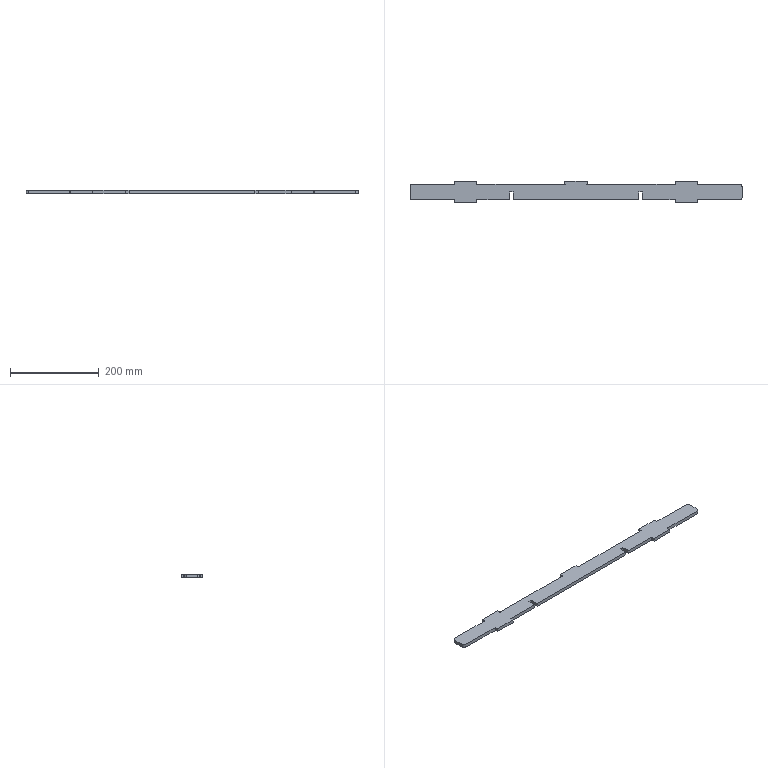Part | SolidWorks | features Fillet 2, FlatPattern 1, ICE 1, SMBaseFlange 1, SheetMetal 1 | 1 solid | 72 faces | box 750 x 49.5 x 8 mm | volume 222099 mm3 | cylinder 38 | plane 34 | commonest cylinder face diameters 2 x19 1 x15 10 x4